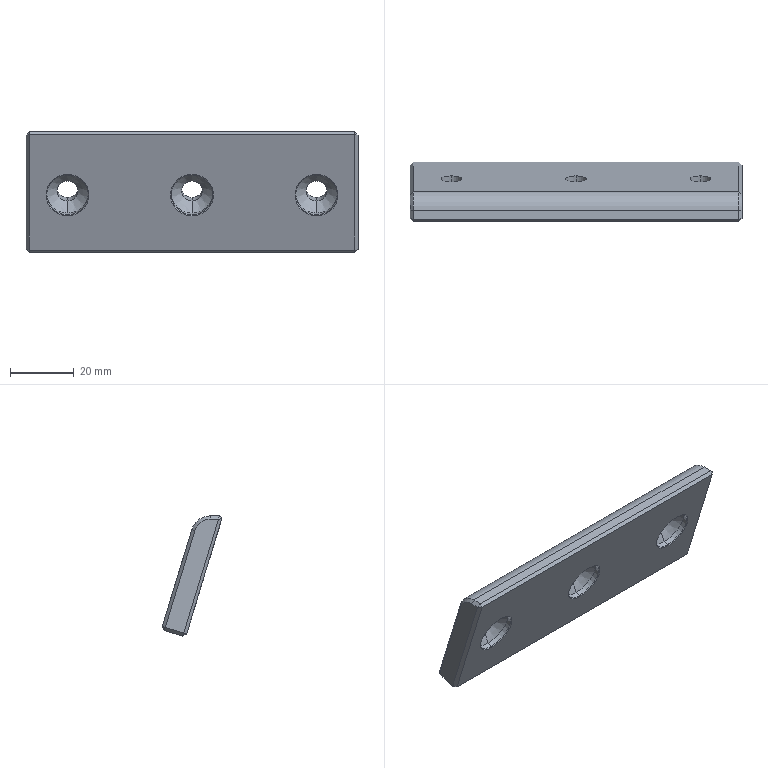Part | Creo | 1 solid | 50 faces | box 104 x 18.672 x 37.672 mm | volume 29709 mm3 | plane 23 | cone 14 | cylinder 13 | commonest cylinder face diameters 6.6 x6 13 x6 12 x1
STEP:
#1=CARTESIAN_POINT('',(0.,0.,0.));
#2=DIRECTION('',(0.,0.,1.));
#3=DIRECTION('',(1.,0.,0.));
#4=AXIS2_PLACEMENT_3D('',#1,#2,#3);
#5=CARTESIAN_POINT('',(38.95,191.692,35.934));
#6=VERTEX_POINT('',#5);
#7=CARTESIAN_POINT('',(38.95,193.621,29.622));
#8=VERTEX_POINT('',#7);
#9=CARTESIAN_POINT('',(38.95,192.656,32.778));
#10=DIRECTION('',(0.,-0.9563,-0.2924));
#11=DIRECTION('',(0.,-0.2924,0.9563));
#12=AXIS2_PLACEMENT_3D('',#9,#10,#11);
#13=CIRCLE('',#12,3.3);
#14=EDGE_CURVE('',#6,#8,#13,.T.);
#15=ORIENTED_EDGE('',*,*,#14,.T.);
#16=CARTESIAN_POINT('',(38.95,190.083,28.54));
#17=VERTEX_POINT('',#16);
#18=CARTESIAN_POINT('',(38.95,190.083,28.54));
#19=DIRECTION('',(0.,0.9563,0.2924));
#20=VECTOR('',#19,3.7);
#21=LINE('',#18,#20);
#22=EDGE_CURVE('',#17,#8,#21,.T.);
#23=ORIENTED_EDGE('',*,*,#22,.F.);
#24=CARTESIAN_POINT('',(38.95,188.153,34.852));
#25=VERTEX_POINT('',#24);
#26=CARTESIAN_POINT('',(38.95,189.118,31.696));
#27=DIRECTION('',(0.,0.9563,0.2924));
#28=DIRECTION('',(0.,0.2924,-0.9563));
#29=AXIS2_PLACEMENT_3D('',#26,#27,#28);
#30=CIRCLE('',#29,3.3);
#31=EDGE_CURVE('',#17,#25,#30,.T.);
#32=ORIENTED_EDGE('',*,*,#31,.T.);
#33=CARTESIAN_POINT('',(38.95,188.153,34.852));
#34=DIRECTION('',(0.,0.9563,0.2924));
#35=VECTOR('',#34,3.7);
#36=LINE('',#33,#35);
#37=EDGE_CURVE('',#25,#6,#36,.T.);
#38=ORIENTED_EDGE('',*,*,#37,.T.);
#39=EDGE_LOOP('',(#15,#23,#32,#38));
#40=FACE_OUTER_BOUND('',#39,.F.);
#41=CARTESIAN_POINT('',(38.95,232.821,45.057));
#42=DIRECTION('',(0.,0.9563,0.2924));
#43=DIRECTION('',(0.,0.2924,-0.9563));
#44=AXIS2_PLACEMENT_3D('',#41,#42,#43);
#45=CYLINDRICAL_SURFACE('',#44,3.3);
#46=ADVANCED_FACE('',(#40),#45,.F.);
#47=CARTESIAN_POINT('',(50.95,188.618,45.987));
#48=VERTEX_POINT('',#47);
#49=CARTESIAN_POINT('',(-51.05,188.618,45.987));
#50=VERTEX_POINT('',#49);
#51=CARTESIAN_POINT('',(50.95,188.618,45.987));
#52=DIRECTION('',(-1.,0.,0.));
#53=VECTOR('',#52,102.);
#54=LINE('',#51,#53);
#55=EDGE_CURVE('',#48,#50,#54,.T.);
#56=ORIENTED_EDGE('',*,*,#55,.T.);
#57=CARTESIAN_POINT('',(-51.05,197.919,15.564));
#58=VERTEX_POINT('',#57);
#59=CARTESIAN_POINT('',(-51.05,197.919,15.564));
#60=DIRECTION('',(0.,-0.2924,0.9563));
#61=VECTOR('',#60,31.813);
#62=LINE('',#59,#61);
#63=EDGE_CURVE('',#58,#50,#62,.T.);
#64=ORIENTED_EDGE('',*,*,#63,.F.);
#65=CARTESIAN_POINT('',(50.95,197.919,15.564));
#66=VERTEX_POINT('',#65);
#67=CARTESIAN_POINT('',(50.95,197.919,15.564));
#68=DIRECTION('',(-1.,0.,0.));
#69=VECTOR('',#68,102.);
#70=LINE('',#67,#69);
#71=EDGE_CURVE('',#66,#58,#70,.T.);
#72=ORIENTED_EDGE('',*,*,#71,.F.);
#73=CARTESIAN_POINT('',(50.95,188.618,45.987));
#74=DIRECTION('',(0.,0.2924,-0.9563));
#75=VECTOR('',#74,31.813);
#76=LINE('',#73,#75);
#77=EDGE_CURVE('',#48,#66,#76,.T.);
#78=ORIENTED_EDGE('',*,*,#77,.F.);
#79=EDGE_LOOP('',(#56,#64,#72,#78));
#80=FACE_OUTER_BOUND('',#79,.F.);
#81=CARTESIAN_POINT('',(-0.05,191.692,35.934));
#82=VERTEX_POINT('',#81);
#83=CARTESIAN_POINT('',(-0.05,193.621,29.622));
#84=VERTEX_POINT('',#83);
#85=CARTESIAN_POINT('',(-0.05,192.656,32.778));
#86=DIRECTION('',(0.,-0.9563,-0.2924));
#87=DIRECTION('',(0.,-0.2924,0.9563));
#88=AXIS2_PLACEMENT_3D('',#85,#86,#87);
#89=CIRCLE('',#88,3.3);
#90=EDGE_CURVE('',#82,#84,#89,.T.);
#91=ORIENTED_EDGE('',*,*,#90,.F.);
#92=CARTESIAN_POINT('',(-0.05,192.656,32.778));
#93=DIRECTION('',(0.,-0.9563,-0.2924));
#94=DIRECTION('',(0.,0.2924,-0.9563));
#95=AXIS2_PLACEMENT_3D('',#92,#93,#94);
#96=CIRCLE('',#95,3.3);
#97=EDGE_CURVE('',#84,#82,#96,.T.);
#98=ORIENTED_EDGE('',*,*,#97,.F.);
#99=EDGE_LOOP('',(#91,#98));
#100=FACE_BOUND('',#99,.F.);
#101=CARTESIAN_POINT('',(-39.05,191.692,35.934));
#102=VERTEX_POINT('',#101);
#103=CARTESIAN_POINT('',(-39.05,193.621,29.622));
#104=VERTEX_POINT('',#103);
#105=CARTESIAN_POINT('',(-39.05,192.656,32.778));
#106=DIRECTION('',(0.,-0.9563,-0.2924));
#107=DIRECTION('',(0.,-0.2924,0.9563));
#108=AXIS2_PLACEMENT_3D('',#105,#106,#107);
#109=CIRCLE('',#108,3.3);
#110=EDGE_CURVE('',#102,#104,#109,.T.);
#111=ORIENTED_EDGE('',*,*,#110,.F.);
#112=CARTESIAN_POINT('',(-39.05,192.656,32.778));
#113=DIRECTION('',(0.,-0.9563,-0.2924));
#114=DIRECTION('',(0.,0.2924,-0.9563));
#115=AXIS2_PLACEMENT_3D('',#112,#113,#114);
#116=CIRCLE('',#115,3.3);
#117=EDGE_CURVE('',#104,#102,#116,.T.);
#118=ORIENTED_EDGE('',*,*,#117,.F.);
#119=EDGE_LOOP('',(#111,#118));
#120=FACE_BOUND('',#119,.F.);
#121=ORIENTED_EDGE('',*,*,#14,.F.);
#122=CARTESIAN_POINT('',(38.95,192.656,32.778));
#123=DIRECTION('',(0.,-0.9563,-0.2924));
#124=DIRECTION('',(0.,0.2924,-0.9563));
#125=AXIS2_PLACEMENT_3D('',#122,#123,#124);
#126=CIRCLE('',#125,3.3);
#127=EDGE_CURVE('',#8,#6,#126,.T.);
#128=ORIENTED_EDGE('',*,*,#127,.F.);
#129=EDGE_LOOP('',(#121,#128));
#130=FACE_BOUND('',#129,.F.);
#131=CARTESIAN_POINT('',(-56.05,205.65,-9.724));
#132=DIRECTION('',(0.,-0.9563,-0.2924));
#133=DIRECTION('',(0.,-0.2924,0.9563));
#134=AXIS2_PLACEMENT_3D('',#131,#132,#133);
#135=PLANE('',#134);
#136=ADVANCED_FACE('',(#80,#100,#120,#130),#135,.F.);
#137=ORIENTED_EDGE('',*,*,#127,.T.);
#138=ORIENTED_EDGE('',*,*,#37,.F.);
#139=CARTESIAN_POINT('',(38.95,189.118,31.696));
#140=DIRECTION('',(0.,0.9563,0.2924));
#141=DIRECTION('',(0.,-0.2924,0.9563));
#142=AXIS2_PLACEMENT_3D('',#139,#140,#141);
#143=CIRCLE('',#142,3.3);
#144=EDGE_CURVE('',#25,#17,#143,.T.);
#145=ORIENTED_EDGE('',*,*,#144,.T.);
#146=ORIENTED_EDGE('',*,*,#22,.T.);
#147=EDGE_LOOP('',(#137,#138,#145,#146));
#148=FACE_OUTER_BOUND('',#147,.F.);
#149=CARTESIAN_POINT('',(38.95,232.821,45.057));
#150=DIRECTION('',(0.,0.9563,0.2924));
#151=DIRECTION('',(0.,0.2924,-0.9563));
#152=AXIS2_PLACEMENT_3D('',#149,#150,#151);
#153=CYLINDRICAL_SURFACE('',#152,3.3);
#154=ADVANCED_FACE('',(#148),#153,.F.);
#155=CARTESIAN_POINT('',(38.95,188.57,24.732));
#156=VERTEX_POINT('',#155);
#157=CARTESIAN_POINT('',(38.95,184.77,37.164));
#158=VERTEX_POINT('',#157);
#159=CARTESIAN_POINT('',(38.95,186.67,30.948));
#160=DIRECTION('',(0.,-0.9563,-0.2924));
#161=DIRECTION('',(0.,0.2924,-0.9563));
#162=AXIS2_PLACEMENT_3D('',#159,#160,#161);
#163=CIRCLE('',#162,6.5);
#164=EDGE_CURVE('',#156,#158,#163,.T.);
#165=ORIENTED_EDGE('',*,*,#164,.F.);
#166=CARTESIAN_POINT('',(38.95,190.083,28.54));
#167=DIRECTION('',(0.,-0.3691,-0.9294));
#168=VECTOR('',#167,4.098);
#169=LINE('',#166,#168);
#170=EDGE_CURVE('',#17,#156,#169,.T.);
#171=ORIENTED_EDGE('',*,*,#170,.F.);
#172=ORIENTED_EDGE('',*,*,#144,.F.);
#173=CARTESIAN_POINT('',(38.95,188.153,34.852));
#174=DIRECTION('',(0.,-0.8257,0.5641));
#175=VECTOR('',#174,4.098);
#176=LINE('',#173,#175);
#177=EDGE_CURVE('',#25,#158,#176,.T.);
#178=ORIENTED_EDGE('',*,*,#177,.T.);
#179=EDGE_LOOP('',(#165,#171,#172,#178));
#180=FACE_OUTER_BOUND('',#179,.F.);
#181=CARTESIAN_POINT('',(38.95,187.894,31.322));
#182=DIRECTION('',(0.,-0.9563,-0.2924));
#183=DIRECTION('',(0.,0.2924,-0.9563));
#184=AXIS2_PLACEMENT_3D('',#181,#182,#183);
#185=CONICAL_SURFACE('',#184,4.9,51.34);
#186=ADVANCED_FACE('',(#180),#185,.F.);
#187=ORIENTED_EDGE('',*,*,#164,.T.);
#188=CARTESIAN_POINT('',(38.95,183.345,36.728));
#189=VERTEX_POINT('',#188);
#190=CARTESIAN_POINT('',(38.95,184.77,37.164));
#191=DIRECTION('',(0.,-0.9563,-0.2924));
#192=VECTOR('',#191,1.49);
#193=LINE('',#190,#192);
#194=EDGE_CURVE('',#158,#189,#193,.T.);
#195=ORIENTED_EDGE('',*,*,#194,.T.);
#196=CARTESIAN_POINT('',(38.95,187.145,24.296));
#197=VERTEX_POINT('',#196);
#198=CARTESIAN_POINT('',(38.95,185.245,30.512));
#199=DIRECTION('',(0.,0.9563,0.2924));
#200=DIRECTION('',(0.,-0.2924,0.9563));
#201=AXIS2_PLACEMENT_3D('',#198,#199,#200);
#202=CIRCLE('',#201,6.5);
#203=EDGE_CURVE('',#189,#197,#202,.T.);
#204=ORIENTED_EDGE('',*,*,#203,.T.);
#205=CARTESIAN_POINT('',(38.95,188.57,24.732));
#206=DIRECTION('',(0.,-0.9563,-0.2924));
#207=VECTOR('',#206,1.49);
#208=LINE('',#205,#207);
#209=EDGE_CURVE('',#156,#197,#208,.T.);
#210=ORIENTED_EDGE('',*,*,#209,.F.);
#211=EDGE_LOOP('',(#187,#195,#204,#210));
#212=FACE_OUTER_BOUND('',#211,.F.);
#213=CARTESIAN_POINT('',(38.95,185.006,30.439));
#214=DIRECTION('',(0.,-0.9563,-0.2924));
#215=DIRECTION('',(0.,0.2924,-0.9563));
#216=AXIS2_PLACEMENT_3D('',#213,#214,#215);
#217=CYLINDRICAL_SURFACE('',#216,6.5);
#218=ADVANCED_FACE('',(#212),#217,.F.);
#219=CARTESIAN_POINT('',(38.95,186.67,30.948));
#220=DIRECTION('',(0.,-0.9563,-0.2924));
#221=DIRECTION('',(0.,-0.2924,0.9563));
#222=AXIS2_PLACEMENT_3D('',#219,#220,#221);
#223=CIRCLE('',#222,6.5);
#224=EDGE_CURVE('',#158,#156,#223,.T.);
#225=ORIENTED_EDGE('',*,*,#224,.T.);
#226=ORIENTED_EDGE('',*,*,#209,.T.);
#227=CARTESIAN_POINT('',(38.95,185.245,30.512));
#228=DIRECTION('',(0.,0.9563,0.2924));
#229=DIRECTION('',(0.,0.2924,-0.9563));
#230=AXIS2_PLACEMENT_3D('',#227,#228,#229);
#231=CIRCLE('',#230,6.5);
#232=EDGE_CURVE('',#197,#189,#231,.T.);
#233=ORIENTED_EDGE('',*,*,#232,.T.);
#234=ORIENTED_EDGE('',*,*,#194,.F.);
#235=EDGE_LOOP('',(#225,#226,#233,#234));
#236=FACE_OUTER_BOUND('',#235,.F.);
#237=CARTESIAN_POINT('',(38.95,185.006,30.439));
#238=DIRECTION('',(0.,-0.9563,-0.2924));
#239=DIRECTION('',(0.,0.2924,-0.9563));
#240=AXIS2_PLACEMENT_3D('',#237,#238,#239);
#241=CYLINDRICAL_SURFACE('',#240,6.5);
#242=ADVANCED_FACE('',(#236),#241,.F.);
#243=ORIENTED_EDGE('',*,*,#224,.F.);
#244=ORIENTED_EDGE('',*,*,#177,.F.);
#245=ORIENTED_EDGE('',*,*,#31,.F.);
#246=ORIENTED_EDGE('',*,*,#170,.T.);
#247=EDGE_LOOP('',(#243,#244,#245,#246));
#248=FACE_OUTER_BOUND('',#247,.F.);
#249=CARTESIAN_POINT('',(38.95,187.894,31.322));
#250=DIRECTION('',(0.,-0.9563,-0.2924));
#251=DIRECTION('',(0.,0.2924,-0.9563));
#252=AXIS2_PLACEMENT_3D('',#249,#250,#251);
#253=CONICAL_SURFACE('',#252,4.9,51.34);
#254=ADVANCED_FACE('',(#248),#253,.F.);
#255=CARTESIAN_POINT('',(38.95,186.979,23.984));
#256=VERTEX_POINT('',#255);
#257=CARTESIAN_POINT('',(38.95,183.032,36.894));
#258=VERTEX_POINT('',#257);
#259=CARTESIAN_POINT('',(38.95,185.006,30.439));
#260=DIRECTION('',(0.,0.9563,0.2924));
#261=DIRECTION('',(0.,0.2924,-0.9563));
#262=AXIS2_PLACEMENT_3D('',#259,#260,#261);
#263=CIRCLE('',#262,6.75);
#264=EDGE_CURVE('',#256,#258,#263,.T.);
#265=ORIENTED_EDGE('',*,*,#264,.T.);
#266=CARTESIAN_POINT('',(38.95,183.345,36.728));
#267=DIRECTION('',(0.,-0.8829,0.4695));
#268=VECTOR('',#267,0.3536);
#269=LINE('',#266,#268);
#270=EDGE_CURVE('',#189,#258,#269,.T.);
#271=ORIENTED_EDGE('',*,*,#270,.F.);
#272=ORIENTED_EDGE('',*,*,#232,.F.);
#273=CARTESIAN_POINT('',(38.95,187.145,24.296));
#274=DIRECTION('',(0.,-0.4695,-0.8829));
#275=VECTOR('',#274,0.3536);
#276=LINE('',#273,#275);
#277=EDGE_CURVE('',#197,#256,#276,.T.);
#278=ORIENTED_EDGE('',*,*,#277,.T.);
#279=EDGE_LOOP('',(#265,#271,#272,#278));
#280=FACE_OUTER_BOUND('',#279,.F.);
#281=CARTESIAN_POINT('',(38.95,185.126,30.475));
#282=DIRECTION('',(0.,-0.9563,-0.2924));
#283=DIRECTION('',(0.,-0.2924,0.9563));
#284=AXIS2_PLACEMENT_3D('',#281,#282,#283);
#285=CONICAL_SURFACE('',#284,6.625,45.);
#286=ADVANCED_FACE('',(#280),#285,.F.);
#287=CARTESIAN_POINT('',(50.95,190.269,13.225));
#288=VERTEX_POINT('',#287);
#289=CARTESIAN_POINT('',(50.95,179.247,49.277));
#290=VERTEX_POINT('',#289);
#291=CARTESIAN_POINT('',(50.95,190.269,13.225));
#292=DIRECTION('',(0.,-0.2924,0.9563));
#293=VECTOR('',#292,37.699);
#294=LINE('',#291,#293);
#295=EDGE_CURVE('',#288,#290,#294,.T.);
#296=ORIENTED_EDGE('',*,*,#295,.F.);
#297=CARTESIAN_POINT('',(-51.05,190.269,13.225));
#298=VERTEX_POINT('',#297);
#299=CARTESIAN_POINT('',(-51.05,190.269,13.225));
#300=DIRECTION('',(1.,0.,0.));
#301=VECTOR('',#300,102.);
#302=LINE('',#299,#301);
#303=EDGE_CURVE('',#298,#288,#302,.T.);
#304=ORIENTED_EDGE('',*,*,#303,.F.);
#305=CARTESIAN_POINT('',(-51.05,179.247,49.277));
#306=VERTEX_POINT('',#305);
#307=CARTESIAN_POINT('',(-51.05,179.247,49.277));
#308=DIRECTION('',(0.,0.2924,-0.9563));
#309=VECTOR('',#308,37.699);
#310=LINE('',#307,#309);
#311=EDGE_CURVE('',#306,#298,#310,.T.);
#312=ORIENTED_EDGE('',*,*,#311,.F.);
#313=CARTESIAN_POINT('',(50.95,179.247,49.277));
#314=DIRECTION('',(-1.,0.,0.));
#315=VECTOR('',#314,102.);
#316=LINE('',#313,#315);
#317=EDGE_CURVE('',#290,#306,#316,.T.);
#318=ORIENTED_EDGE('',*,*,#317,.F.);
#319=EDGE_LOOP('',(#296,#304,#312,#318));
#320=FACE_OUTER_BOUND('',#319,.F.);
#321=ORIENTED_EDGE('',*,*,#264,.F.);
#322=CARTESIAN_POINT('',(38.95,185.006,30.439));
#323=DIRECTION('',(0.,0.9563,0.2924));
#324=DIRECTION('',(0.,-0.2924,0.9563));
#325=AXIS2_PLACEMENT_3D('',#322,#323,#324);
#326=CIRCLE('',#325,6.75);
#327=EDGE_CURVE('',#258,#256,#326,.T.);
#328=ORIENTED_EDGE('',*,*,#327,.F.);
#329=EDGE_LOOP('',(#321,#328));
#330=FACE_BOUND('',#329,.F.);
#331=CARTESIAN_POINT('',(-0.05,186.979,23.984));
#332=VERTEX_POINT('',#331);
#333=CARTESIAN_POINT('',(-0.05,183.032,36.894));
#334=VERTEX_POINT('',#333);
#335=CARTESIAN_POINT('',(-0.05,185.006,30.439));
#336=DIRECTION('',(0.,0.9563,0.2924));
#337=DIRECTION('',(0.,0.2924,-0.9563));
#338=AXIS2_PLACEMENT_3D('',#335,#336,#337);
#339=CIRCLE('',#338,6.75);
#340=EDGE_CURVE('',#332,#334,#339,.T.);
#341=ORIENTED_EDGE('',*,*,#340,.F.);
#342=CARTESIAN_POINT('',(-0.05,185.006,30.439));
#343=DIRECTION('',(0.,0.9563,0.2924));
#344=DIRECTION('',(0.,-0.2924,0.9563));
#345=AXIS2_PLACEMENT_3D('',#342,#343,#344);
#346=CIRCLE('',#345,6.75);
#347=EDGE_CURVE('',#334,#332,#346,.T.);
#348=ORIENTED_EDGE('',*,*,#347,.F.);
#349=EDGE_LOOP('',(#341,#348));
#350=FACE_BOUND('',#349,.F.);
#351=CARTESIAN_POINT('',(-39.05,186.979,23.984));
#352=VERTEX_POINT('',#351);
#353=CARTESIAN_POINT('',(-39.05,183.032,36.894));
#354=VERTEX_POINT('',#353);
#355=CARTESIAN_POINT('',(-39.05,185.006,30.439));
#356=DIRECTION('',(0.,0.9563,0.2924));
#357=DIRECTION('',(0.,0.2924,-0.9563));
#358=AXIS2_PLACEMENT_3D('',#355,#356,#357);
#359=CIRCLE('',#358,6.75);
#360=EDGE_CURVE('',#352,#354,#359,.T.);
#361=ORIENTED_EDGE('',*,*,#360,.F.);
#362=CARTESIAN_POINT('',(-39.05,185.006,30.439));
#363=DIRECTION('',(0.,0.9563,0.2924));
#364=DIRECTION('',(0.,-0.2924,0.9563));
#365=AXIS2_PLACEMENT_3D('',#362,#363,#364);
#366=CIRCLE('',#365,6.75);
#367=EDGE_CURVE('',#354,#352,#366,.T.);
#368=ORIENTED_EDGE('',*,*,#367,.F.);
#369=EDGE_LOOP('',(#361,#368));
#370=FACE_BOUND('',#369,.F.);
#371=CARTESIAN_POINT('',(-56.05,198.,-12.063));
#372=DIRECTION('',(0.,-0.9563,-0.2924));
#373=DIRECTION('',(0.,-0.2924,0.9563));
#374=AXIS2_PLACEMENT_3D('',#371,#372,#373);
#375=PLANE('',#374);
#376=ADVANCED_FACE('',(#320,#330,#350,#370),#375,.T.);
#377=CARTESIAN_POINT('',(51.95,180.306,49.233));
#378=VERTEX_POINT('',#377);
#379=CARTESIAN_POINT('',(51.95,180.306,49.233));
#380=DIRECTION('',(-0.6862,-0.7268,0.02999));
#381=VECTOR('',#380,1.457);
#382=LINE('',#379,#381);
#383=EDGE_CURVE('',#378,#290,#382,.T.);
#384=ORIENTED_EDGE('',*,*,#383,.F.);
#385=CARTESIAN_POINT('',(51.95,191.225,13.518));
#386=VERTEX_POINT('',#385);
#387=CARTESIAN_POINT('',(51.95,180.306,49.233));
#388=DIRECTION('',(0.,0.2924,-0.9563));
#389=VECTOR('',#388,37.347);
#390=LINE('',#387,#389);
#391=EDGE_CURVE('',#378,#386,#390,.T.);
#392=ORIENTED_EDGE('',*,*,#391,.T.);
#393=CARTESIAN_POINT('',(51.95,191.225,13.518));
#394=DIRECTION('',(-0.7071,-0.6762,-0.2067));
#395=VECTOR('',#394,1.414);
#396=LINE('',#393,#395);
#397=EDGE_CURVE('',#386,#288,#396,.T.);
#398=ORIENTED_EDGE('',*,*,#397,.T.);
#399=ORIENTED_EDGE('',*,*,#295,.T.);
#400=EDGE_LOOP('',(#384,#392,#398,#399));
#401=FACE_OUTER_BOUND('',#400,.F.);
#402=CARTESIAN_POINT('',(50.95,198.,-12.063));
#403=DIRECTION('',(0.7071,-0.6762,-0.2067));
#404=DIRECTION('',(0.,-0.2924,0.9563));
#405=AXIS2_PLACEMENT_3D('',#402,#403,#404);
#406=PLANE('',#405);
#407=ADVANCED_FACE('',(#401),#406,.T.);
#408=CARTESIAN_POINT('',(50.95,179.954,50.233));
#409=VERTEX_POINT('',#408);
#410=CARTESIAN_POINT('',(50.95,179.954,50.233));
#411=DIRECTION('',(0.,-0.5948,-0.8039));
#412=VECTOR('',#411,1.19);
#413=LINE('',#410,#412);
#414=EDGE_CURVE('',#409,#290,#413,.T.);
#415=ORIENTED_EDGE('',*,*,#414,.F.);
#416=CARTESIAN_POINT('',(51.95,180.306,49.233));
#417=DIRECTION('',(-0.6862,-0.2412,0.6862));
#418=VECTOR('',#417,1.457);
#419=LINE('',#416,#418);
#420=EDGE_CURVE('',#378,#409,#419,.T.);
#421=ORIENTED_EDGE('',*,*,#420,.F.);
#422=ORIENTED_EDGE('',*,*,#383,.T.);
#423=EDGE_LOOP('',(#415,#421,#422));
#424=FACE_OUTER_BOUND('',#423,.F.);
#425=CARTESIAN_POINT('',(50.95,179.954,50.233));
#426=DIRECTION('',(0.6595,-0.6043,0.4471));
#427=DIRECTION('',(-0.6756,-0.7373,0.));
#428=AXIS2_PLACEMENT_3D('',#425,#426,#427);
#429=PLANE('',#428);
#430=ADVANCED_FACE('',(#424),#429,.T.);
#431=CARTESIAN_POINT('',(-51.05,179.954,50.233));
#432=VERTEX_POINT('',#431);
#433=CARTESIAN_POINT('',(-51.05,179.247,49.277));
#434=DIRECTION('',(0.,0.5948,0.8039));
#435=VECTOR('',#434,1.19);
#436=LINE('',#433,#435);
#437=EDGE_CURVE('',#306,#432,#436,.T.);
#438=ORIENTED_EDGE('',*,*,#437,.T.);
#439=CARTESIAN_POINT('',(-51.05,179.954,50.233));
#440=DIRECTION('',(1.,0.,0.));
#441=VECTOR('',#440,102.);
#442=LINE('',#439,#441);
#443=EDGE_CURVE('',#432,#409,#442,.T.);
#444=ORIENTED_EDGE('',*,*,#443,.T.);
#445=ORIENTED_EDGE('',*,*,#414,.T.);
#446=ORIENTED_EDGE('',*,*,#317,.T.);
#447=EDGE_LOOP('',(#438,#444,#445,#446));
#448=FACE_OUTER_BOUND('',#447,.F.);
#449=CARTESIAN_POINT('',(-56.05,179.247,49.277));
#450=DIRECTION('',(0.,-0.8039,0.5948));
#451=DIRECTION('',(-1.,0.,0.));
#452=AXIS2_PLACEMENT_3D('',#449,#450,#451);
#453=PLANE('',#452);
#454=ADVANCED_FACE('',(#448),#453,.T.);
#455=CARTESIAN_POINT('',(-52.05,180.306,49.233));
#456=VERTEX_POINT('',#455);
#457=CARTESIAN_POINT('',(-51.05,179.247,49.277));
#458=DIRECTION('',(-0.6862,0.7268,-0.02999));
#459=VECTOR('',#458,1.457);
#460=LINE('',#457,#459);
#461=EDGE_CURVE('',#306,#456,#460,.T.);
#462=ORIENTED_EDGE('',*,*,#461,.T.);
#463=CARTESIAN_POINT('',(-51.05,179.954,50.233));
#464=DIRECTION('',(-0.6862,0.2412,-0.6862));
#465=VECTOR('',#464,1.457);
#466=LINE('',#463,#465);
#467=EDGE_CURVE('',#432,#456,#466,.T.);
#468=ORIENTED_EDGE('',*,*,#467,.F.);
#469=ORIENTED_EDGE('',*,*,#437,.F.);
#470=EDGE_LOOP('',(#462,#468,#469));
#471=FACE_OUTER_BOUND('',#470,.F.);
#472=CARTESIAN_POINT('',(-52.05,180.306,49.233));
#473=DIRECTION('',(-0.6595,-0.6043,0.4471));
#474=DIRECTION('',(-0.6756,0.7373,0.));
#475=AXIS2_PLACEMENT_3D('',#472,#473,#474);
#476=PLANE('',#475);
#477=ADVANCED_FACE('',(#471),#476,.T.);
#478=ORIENTED_EDGE('',*,*,#461,.F.);
#479=ORIENTED_EDGE('',*,*,#311,.T.);
#480=CARTESIAN_POINT('',(-52.05,191.225,13.518));
#481=VERTEX_POINT('',#480);
#482=CARTESIAN_POINT('',(-51.05,190.269,13.225));
#483=DIRECTION('',(-0.7071,0.6762,0.2067));
#484=VECTOR('',#483,1.414);
#485=LINE('',#482,#484);
#486=EDGE_CURVE('',#298,#481,#485,.T.);
#487=ORIENTED_EDGE('',*,*,#486,.T.);
#488=CARTESIAN_POINT('',(-52.05,191.225,13.518));
#489=DIRECTION('',(0.,-0.2924,0.9563));
#490=VECTOR('',#489,37.347);
#491=LINE('',#488,#490);
#492=EDGE_CURVE('',#481,#456,#491,.T.);
#493=ORIENTED_EDGE('',*,*,#492,.T.);
#494=EDGE_LOOP('',(#478,#479,#487,#493));
#495=FACE_OUTER_BOUND('',#494,.F.);
#496=CARTESIAN_POINT('',(-51.05,198.,-12.063));
#497=DIRECTION('',(0.7071,0.6762,0.2067));
#498=DIRECTION('',(0.,-0.2924,0.9563));
#499=AXIS2_PLACEMENT_3D('',#496,#497,#498);
#500=PLANE('',#499);
#501=ADVANCED_FACE('',(#495),#500,.F.);
#502=CARTESIAN_POINT('',(-51.05,191.517,12.561));
#503=VERTEX_POINT('',#502);
#504=CARTESIAN_POINT('',(-52.05,191.225,13.518));
#505=DIRECTION('',(0.7071,0.2067,-0.6762));
#506=VECTOR('',#505,1.414);
#507=LINE('',#504,#506);
#508=EDGE_CURVE('',#481,#503,#507,.T.);
#509=ORIENTED_EDGE('',*,*,#508,.F.);
#510=ORIENTED_EDGE('',*,*,#486,.F.);
#511=CARTESIAN_POINT('',(-51.05,191.517,12.561));
#512=DIRECTION('',(0.,-0.8829,0.4695));
#513=VECTOR('',#512,1.414);
#514=LINE('',#511,#513);
#515=EDGE_CURVE('',#503,#298,#514,.T.);
#516=ORIENTED_EDGE('',*,*,#515,.F.);
#517=EDGE_LOOP('',(#509,#510,#516));
#518=FACE_OUTER_BOUND('',#517,.F.);
#519=CARTESIAN_POINT('',(-51.05,190.269,13.225));
#520=DIRECTION('',(-0.5774,-0.3833,-0.7209));
#521=DIRECTION('',(-0.7805,0.,0.6251));
#522=AXIS2_PLACEMENT_3D('',#519,#520,#521);
#523=PLANE('',#522);
#524=ADVANCED_FACE('',(#518),#523,.T.);
#525=CARTESIAN_POINT('',(-51.05,197.255,14.316));
#526=VERTEX_POINT('',#525);
#527=CARTESIAN_POINT('',(-52.05,196.963,15.272));
#528=VERTEX_POINT('',#527);
#529=CARTESIAN_POINT('',(-51.05,197.255,14.316));
#530=DIRECTION('',(-0.7071,-0.2067,0.6762));
#531=VECTOR('',#530,1.414);
#532=LINE('',#529,#531);
#533=EDGE_CURVE('',#526,#528,#532,.T.);
#534=ORIENTED_EDGE('',*,*,#533,.T.);
#535=CARTESIAN_POINT('',(-52.05,196.963,15.272));
#536=DIRECTION('',(0.,-0.9563,-0.2924));
#537=VECTOR('',#536,6.);
#538=LINE('',#535,#537);
#539=EDGE_CURVE('',#528,#481,#538,.T.);
#540=ORIENTED_EDGE('',*,*,#539,.T.);
#541=ORIENTED_EDGE('',*,*,#508,.T.);
#542=CARTESIAN_POINT('',(-51.05,191.517,12.561));
#543=DIRECTION('',(0.,0.9563,0.2924));
#544=VECTOR('',#543,6.);
#545=LINE('',#542,#544);
#546=EDGE_CURVE('',#503,#526,#545,.T.);
#547=ORIENTED_EDGE('',*,*,#546,.T.);
#548=EDGE_LOOP('',(#534,#540,#541,#547));
#549=FACE_OUTER_BOUND('',#548,.F.);
#550=CARTESIAN_POINT('',(-52.05,190.269,13.225));
#551=DIRECTION('',(0.7071,-0.2067,0.6762));
#552=DIRECTION('',(0.,0.9563,0.2924));
#553=AXIS2_PLACEMENT_3D('',#550,#551,#552);
#554=PLANE('',#553);
#555=ADVANCED_FACE('',(#549),#554,.F.);
#556=CARTESIAN_POINT('',(-52.05,196.963,15.272));
#557=DIRECTION('',(0.7071,0.6762,0.2067));
#558=VECTOR('',#557,1.414);
#559=LINE('',#556,#558);
#560=EDGE_CURVE('',#528,#58,#559,.T.);
#561=ORIENTED_EDGE('',*,*,#560,.F.);
#562=ORIENTED_EDGE('',*,*,#533,.F.);
#563=CARTESIAN_POINT('',(-51.05,197.919,15.564));
#564=DIRECTION('',(0.,-0.4695,-0.8829));
#565=VECTOR('',#564,1.414);
#566=LINE('',#563,#565);
#567=EDGE_CURVE('',#58,#526,#566,.T.);
#568=ORIENTED_EDGE('',*,*,#567,.F.);
#569=EDGE_LOOP('',(#561,#562,#568));
#570=FACE_OUTER_BOUND('',#569,.F.);
#571=CARTESIAN_POINT('',(-51.05,197.919,15.564));
#572=DIRECTION('',(-0.5774,0.7209,-0.3833));
#573=DIRECTION('',(0.7805,0.6251,0.));
#574=AXIS2_PLACEMENT_3D('',#571,#572,#573);
#575=PLANE('',#574);
#576=ADVANCED_FACE('',(#570),#575,.T.);
#577=CARTESIAN_POINT('',(-52.05,187.662,45.695));
#578=VERTEX_POINT('',#577);
#579=CARTESIAN_POINT('',(-51.05,188.618,45.987));
#580=DIRECTION('',(-0.7071,-0.6762,-0.2067));
#581=VECTOR('',#580,1.414);
#582=LINE('',#579,#581);
#583=EDGE_CURVE('',#50,#578,#582,.T.);
#584=ORIENTED_EDGE('',*,*,#583,.T.);
#585=CARTESIAN_POINT('',(-52.05,187.662,45.695));
#586=DIRECTION('',(0.,0.2924,-0.9563));
#587=VECTOR('',#586,31.813);
#588=LINE('',#585,#587);
#589=EDGE_CURVE('',#578,#528,#588,.T.);
#590=ORIENTED_EDGE('',*,*,#589,.T.);
#591=ORIENTED_EDGE('',*,*,#560,.T.);
#592=ORIENTED_EDGE('',*,*,#63,.T.);
#593=EDGE_LOOP('',(#584,#590,#591,#592));
#594=FACE_OUTER_BOUND('',#593,.F.);
#595=CARTESIAN_POINT('',(-52.05,187.379,46.619));
#596=DIRECTION('',(-0.7071,0.6762,0.2067));
#597=DIRECTION('',(0.,0.2924,-0.9563));
#598=AXIS2_PLACEMENT_3D('',#595,#596,#597);
#599=PLANE('',#598);
#600=ADVANCED_FACE('',(#594),#599,.T.);
#601=CARTESIAN_POINT('',(-52.05,182.88,49.233));
#602=VERTEX_POINT('',#601);
#603=CARTESIAN_POINT('',(-51.05,182.88,50.233));
#604=VERTEX_POINT('',#603);
#605=CARTESIAN_POINT('',(-52.05,182.88,49.233));
#606=DIRECTION('',(0.7071,0.,0.7071));
#607=VECTOR('',#606,1.414);
#608=LINE('',#605,#607);
#609=EDGE_CURVE('',#602,#604,#608,.T.);
#610=ORIENTED_EDGE('',*,*,#609,.F.);
#611=CARTESIAN_POINT('',(-52.05,182.88,44.233));
#612=DIRECTION('',(-1.,0.,0.));
#613=DIRECTION('',(0.,0.,1.));
#614=AXIS2_PLACEMENT_3D('',#611,#612,#613);
#615=CIRCLE('',#614,5.);
#616=EDGE_CURVE('',#602,#578,#615,.T.);
#617=ORIENTED_EDGE('',*,*,#616,.T.);
#618=ORIENTED_EDGE('',*,*,#583,.F.);
#619=CARTESIAN_POINT('',(-51.05,182.88,44.233));
#620=DIRECTION('',(-1.,0.,0.));
#621=DIRECTION('',(0.,0.,1.));
#622=AXIS2_PLACEMENT_3D('',#619,#620,#621);
#623=CIRCLE('',#622,6.);
#624=EDGE_CURVE('',#604,#50,#623,.T.);
#625=ORIENTED_EDGE('',*,*,#624,.F.);
#626=EDGE_LOOP('',(#610,#617,#618,#625));
#627=FACE_OUTER_BOUND('',#626,.F.);
#628=CARTESIAN_POINT('',(-51.55,182.88,44.233));
#629=DIRECTION('',(1.,0.,0.));
#630=DIRECTION('',(0.,0.,-1.));
#631=AXIS2_PLACEMENT_3D('',#628,#629,#630);
#632=CONICAL_SURFACE('',#631,5.5,45.);
#633=ADVANCED_FACE('',(#627),#632,.T.);
#634=ORIENTED_EDGE('',*,*,#467,.T.);
#635=CARTESIAN_POINT('',(-52.05,180.306,49.233));
#636=DIRECTION('',(0.,1.,0.));
#637=VECTOR('',#636,2.574);
#638=LINE('',#635,#637);
#639=EDGE_CURVE('',#456,#602,#638,.T.);
#640=ORIENTED_EDGE('',*,*,#639,.T.);
#641=ORIENTED_EDGE('',*,*,#609,.T.);
#642=CARTESIAN_POINT('',(-51.05,182.88,50.233));
#643=DIRECTION('',(0.,-1.,0.));
#644=VECTOR('',#643,2.926);
#645=LINE('',#642,#644);
#646=EDGE_CURVE('',#604,#432,#645,.T.);
#647=ORIENTED_EDGE('',*,*,#646,.T.);
#648=EDGE_LOOP('',(#634,#640,#641,#647));
#649=FACE_OUTER_BOUND('',#648,.F.);
#650=CARTESIAN_POINT('',(-51.05,168.954,50.233));
#651=DIRECTION('',(-0.7071,0.,0.7071));
#652=DIRECTION('',(0.,-1.,0.));
#653=AXIS2_PLACEMENT_3D('',#650,#651,#652);
#654=PLANE('',#653);
#655=ADVANCED_FACE('',(#649),#654,.T.);
#656=ORIENTED_EDGE('',*,*,#589,.F.);
#657=ORIENTED_EDGE('',*,*,#616,.F.);
#658=ORIENTED_EDGE('',*,*,#639,.F.);
#659=ORIENTED_EDGE('',*,*,#492,.F.);
#660=ORIENTED_EDGE('',*,*,#539,.F.);
#661=EDGE_LOOP('',(#656,#657,#658,#659,#660));
#662=FACE_OUTER_BOUND('',#661,.F.);
#663=CARTESIAN_POINT('',(-52.05,180.685,44.572));
#664=DIRECTION('',(-1.,0.,0.));
#665=DIRECTION('',(0.,-0.2924,0.9563));
#666=AXIS2_PLACEMENT_3D('',#663,#664,#665);
#667=PLANE('',#666);
#668=ADVANCED_FACE('',(#662),#667,.T.);
#669=ORIENTED_EDGE('',*,*,#443,.F.);
#670=ORIENTED_EDGE('',*,*,#646,.F.);
#671=CARTESIAN_POINT('',(50.95,182.88,50.233));
#672=VERTEX_POINT('',#671);
#673=CARTESIAN_POINT('',(-51.05,182.88,50.233));
#674=DIRECTION('',(1.,0.,0.));
#675=VECTOR('',#674,102.);
#676=LINE('',#673,#675);
#677=EDGE_CURVE('',#604,#672,#676,.T.);
#678=ORIENTED_EDGE('',*,*,#677,.T.);
#679=CARTESIAN_POINT('',(50.95,179.954,50.233));
#680=DIRECTION('',(0.,1.,0.));
#681=VECTOR('',#680,2.926);
#682=LINE('',#679,#681);
#683=EDGE_CURVE('',#409,#672,#682,.T.);
#684=ORIENTED_EDGE('',*,*,#683,.F.);
#685=EDGE_LOOP('',(#669,#670,#678,#684));
#686=FACE_OUTER_BOUND('',#685,.F.);
#687=CARTESIAN_POINT('',(-56.05,168.954,50.233));
#688=DIRECTION('',(0.,0.,-1.));
#689=DIRECTION('',(0.,-1.,0.));
#690=AXIS2_PLACEMENT_3D('',#687,#688,#689);
#691=PLANE('',#690);
#692=ADVANCED_FACE('',(#686),#691,.F.);
#693=ORIENTED_EDGE('',*,*,#677,.F.);
#694=ORIENTED_EDGE('',*,*,#624,.T.);
#695=ORIENTED_EDGE('',*,*,#55,.F.);
#696=CARTESIAN_POINT('',(50.95,182.88,44.233));
#697=DIRECTION('',(1.,0.,0.));
#698=DIRECTION('',(0.,0.9563,0.2924));
#699=AXIS2_PLACEMENT_3D('',#696,#697,#698);
#700=CIRCLE('',#699,6.);
#701=EDGE_CURVE('',#48,#672,#700,.T.);
#702=ORIENTED_EDGE('',*,*,#701,.T.);
#703=EDGE_LOOP('',(#693,#694,#695,#702));
#704=FACE_OUTER_BOUND('',#703,.F.);
#705=CARTESIAN_POINT('',(-56.05,182.88,44.233));
#706=DIRECTION('',(1.,0.,0.));
#707=DIRECTION('',(0.,0.,-1.));
#708=AXIS2_PLACEMENT_3D('',#705,#706,#707);
#709=CYLINDRICAL_SURFACE('',#708,6.);
#710=ADVANCED_FACE('',(#704),#709,.T.);
#711=CARTESIAN_POINT('',(51.95,182.88,49.233));
#712=VERTEX_POINT('',#711);
#713=CARTESIAN_POINT('',(50.95,182.88,50.233));
#714=DIRECTION('',(0.7071,0.,-0.7071));
#715=VECTOR('',#714,1.414);
#716=LINE('',#713,#715);
#717=EDGE_CURVE('',#672,#712,#716,.T.);
#718=ORIENTED_EDGE('',*,*,#717,.F.);
#719=ORIENTED_EDGE('',*,*,#701,.F.);
#720=CARTESIAN_POINT('',(51.95,187.662,45.695));
#721=VERTEX_POINT('',#720);
#722=CARTESIAN_POINT('',(51.95,187.662,45.695));
#723=DIRECTION('',(-0.7071,0.6762,0.2067));
#724=VECTOR('',#723,1.414);
#725=LINE('',#722,#724);
#726=EDGE_CURVE('',#721,#48,#725,.T.);
#727=ORIENTED_EDGE('',*,*,#726,.F.);
#728=CARTESIAN_POINT('',(51.95,182.88,44.233));
#729=DIRECTION('',(1.,0.,0.));
#730=DIRECTION('',(0.,0.9563,0.2924));
#731=AXIS2_PLACEMENT_3D('',#728,#729,#730);
#732=CIRCLE('',#731,5.);
#733=EDGE_CURVE('',#721,#712,#732,.T.);
#734=ORIENTED_EDGE('',*,*,#733,.T.);
#735=EDGE_LOOP('',(#718,#719,#727,#734));
#736=FACE_OUTER_BOUND('',#735,.F.);
#737=CARTESIAN_POINT('',(51.45,182.88,44.233));
#738=DIRECTION('',(-1.,0.,0.));
#739=DIRECTION('',(0.,0.,1.));
#740=AXIS2_PLACEMENT_3D('',#737,#738,#739);
#741=CONICAL_SURFACE('',#740,5.5,45.);
#742=ADVANCED_FACE('',(#736),#741,.T.);
#743=ORIENTED_EDGE('',*,*,#420,.T.);
#744=ORIENTED_EDGE('',*,*,#683,.T.);
#745=ORIENTED_EDGE('',*,*,#717,.T.);
#746=CARTESIAN_POINT('',(51.95,182.88,49.233));
#747=DIRECTION('',(0.,-1.,0.));
#748=VECTOR('',#747,2.574);
#749=LINE('',#746,#748);
#750=EDGE_CURVE('',#712,#378,#749,.T.);
#751=ORIENTED_EDGE('',*,*,#750,.T.);
#752=EDGE_LOOP('',(#743,#744,#745,#751));
#753=FACE_OUTER_BOUND('',#752,.F.);
#754=CARTESIAN_POINT('',(51.95,198.,49.233));
#755=DIRECTION('',(-0.7071,0.,-0.7071));
#756=DIRECTION('',(0.,1.,0.));
#757=AXIS2_PLACEMENT_3D('',#754,#755,#756);
#758=PLANE('',#757);
#759=ADVANCED_FACE('',(#753),#758,.F.);
#760=ORIENTED_EDGE('',*,*,#391,.F.);
#761=ORIENTED_EDGE('',*,*,#750,.F.);
#762=ORIENTED_EDGE('',*,*,#733,.F.);
#763=CARTESIAN_POINT('',(51.95,196.963,15.272));
#764=VERTEX_POINT('',#763);
#765=CARTESIAN_POINT('',(51.95,196.963,15.272));
#766=DIRECTION('',(0.,-0.2924,0.9563));
#767=VECTOR('',#766,31.813);
#768=LINE('',#765,#767);
#769=EDGE_CURVE('',#764,#721,#768,.T.);
#770=ORIENTED_EDGE('',*,*,#769,.F.);
#771=CARTESIAN_POINT('',(51.95,191.225,13.518));
#772=DIRECTION('',(0.,0.9563,0.2924));
#773=VECTOR('',#772,6.);
#774=LINE('',#771,#773);
#775=EDGE_CURVE('',#386,#764,#774,.T.);
#776=ORIENTED_EDGE('',*,*,#775,.F.);
#777=EDGE_LOOP('',(#760,#761,#762,#770,#776));
#778=FACE_OUTER_BOUND('',#777,.F.);
#779=CARTESIAN_POINT('',(51.95,198.,-12.063));
#780=DIRECTION('',(-1.,0.,0.));
#781=DIRECTION('',(0.,-0.2924,0.9563));
#782=AXIS2_PLACEMENT_3D('',#779,#780,#781);
#783=PLANE('',#782);
#784=ADVANCED_FACE('',(#778),#783,.F.);
#785=ORIENTED_EDGE('',*,*,#726,.T.);
#786=ORIENTED_EDGE('',*,*,#77,.T.);
#787=CARTESIAN_POINT('',(50.95,197.919,15.564));
#788=DIRECTION('',(0.7071,-0.6762,-0.2067));
#789=VECTOR('',#788,1.414);
#790=LINE('',#787,#789);
#791=EDGE_CURVE('',#66,#764,#790,.T.);
#792=ORIENTED_EDGE('',*,*,#791,.T.);
#793=ORIENTED_EDGE('',*,*,#769,.T.);
#794=EDGE_LOOP('',(#785,#786,#792,#793));
#795=FACE_OUTER_BOUND('',#794,.F.);
#796=CARTESIAN_POINT('',(51.95,204.694,-10.016));
#797=DIRECTION('',(-0.7071,-0.6762,-0.2067));
#798=DIRECTION('',(0.,0.2924,-0.9563));
#799=AXIS2_PLACEMENT_3D('',#796,#797,#798);
#800=PLANE('',#799);
#801=ADVANCED_FACE('',(#795),#800,.F.);
#802=ORIENTED_EDGE('',*,*,#791,.F.);
#803=CARTESIAN_POINT('',(50.95,197.255,14.316));
#804=VERTEX_POINT('',#803);
#805=CARTESIAN_POINT('',(50.95,197.255,14.316));
#806=DIRECTION('',(0.,0.4695,0.8829));
#807=VECTOR('',#806,1.414);
#808=LINE('',#805,#807);
#809=EDGE_CURVE('',#804,#66,#808,.T.);
#810=ORIENTED_EDGE('',*,*,#809,.F.);
#811=CARTESIAN_POINT('',(51.95,196.963,15.272));
#812=DIRECTION('',(-0.7071,0.2067,-0.6762));
#813=VECTOR('',#812,1.414);
#814=LINE('',#811,#813);
#815=EDGE_CURVE('',#764,#804,#814,.T.);
#816=ORIENTED_EDGE('',*,*,#815,.F.);
#817=EDGE_LOOP('',(#802,#810,#816));
#818=FACE_OUTER_BOUND('',#817,.F.);
#819=CARTESIAN_POINT('',(50.95,197.255,14.316));
#820=DIRECTION('',(0.5774,0.7209,-0.3833));
#821=DIRECTION('',(0.7805,-0.6251,0.));
#822=AXIS2_PLACEMENT_3D('',#819,#820,#821);
#823=PLANE('',#822);
#824=ADVANCED_FACE('',(#818),#823,.T.);
#825=ORIENTED_EDGE('',*,*,#567,.T.);
#826=CARTESIAN_POINT('',(-51.05,197.255,14.316));
#827=DIRECTION('',(1.,0.,0.));
#828=VECTOR('',#827,102.);
#829=LINE('',#826,#828);
#830=EDGE_CURVE('',#526,#804,#829,.T.);
#831=ORIENTED_EDGE('',*,*,#830,.T.);
#832=ORIENTED_EDGE('',*,*,#809,.T.);
#833=ORIENTED_EDGE('',*,*,#71,.T.);
#834=EDGE_LOOP('',(#825,#831,#832,#833));
#835=FACE_OUTER_BOUND('',#834,.F.);
#836=CARTESIAN_POINT('',(-54.05,197.255,14.316));
#837=DIRECTION('',(0.,0.8829,-0.4695));
#838=DIRECTION('',(1.,0.,0.));
#839=AXIS2_PLACEMENT_3D('',#836,#837,#838);
#840=PLANE('',#839);
#841=ADVANCED_FACE('',(#835),#840,.T.);
#842=CARTESIAN_POINT('',(50.95,191.517,12.561));
#843=VERTEX_POINT('',#842);
#844=CARTESIAN_POINT('',(50.95,191.517,12.561));
#845=DIRECTION('',(-1.,0.,0.));
#846=VECTOR('',#845,102.);
#847=LINE('',#844,#846);
#848=EDGE_CURVE('',#843,#503,#847,.T.);
#849=ORIENTED_EDGE('',*,*,#848,.F.);
#850=CARTESIAN_POINT('',(50.95,197.255,14.316));
#851=DIRECTION('',(0.,-0.9563,-0.2924));
#852=VECTOR('',#851,6.);
#853=LINE('',#850,#852);
#854=EDGE_CURVE('',#804,#843,#853,.T.);
#855=ORIENTED_EDGE('',*,*,#854,.F.);
#856=ORIENTED_EDGE('',*,*,#830,.F.);
#857=ORIENTED_EDGE('',*,*,#546,.F.);
#858=EDGE_LOOP('',(#849,#855,#856,#857));
#859=FACE_OUTER_BOUND('',#858,.F.);
#860=CARTESIAN_POINT('',(-54.05,190.561,12.269));
#861=DIRECTION('',(0.,0.2924,-0.9563));
#862=DIRECTION('',(-1.,0.,0.));
#863=AXIS2_PLACEMENT_3D('',#860,#861,#862);
#864=PLANE('',#863);
#865=ADVANCED_FACE('',(#859),#864,.T.);
#866=ORIENTED_EDGE('',*,*,#515,.T.);
#867=ORIENTED_EDGE('',*,*,#303,.T.);
#868=CARTESIAN_POINT('',(50.95,190.269,13.225));
#869=DIRECTION('',(0.,0.8829,-0.4695));
#870=VECTOR('',#869,1.414);
#871=LINE('',#868,#870);
#872=EDGE_CURVE('',#288,#843,#871,.T.);
#873=ORIENTED_EDGE('',*,*,#872,.T.);
#874=ORIENTED_EDGE('',*,*,#848,.T.);
#875=EDGE_LOOP('',(#866,#867,#873,#874));
#876=FACE_OUTER_BOUND('',#875,.F.);
#877=CARTESIAN_POINT('',(-56.05,190.269,13.225));
#878=DIRECTION('',(0.,0.4695,0.8829));
#879=DIRECTION('',(-1.,0.,0.));
#880=AXIS2_PLACEMENT_3D('',#877,#878,#879);
#881=PLANE('',#880);
#882=ADVANCED_FACE('',(#876),#881,.F.);
#883=ORIENTED_EDGE('',*,*,#872,.F.);
#884=ORIENTED_EDGE('',*,*,#397,.F.);
#885=CARTESIAN_POINT('',(50.95,191.517,12.561));
#886=DIRECTION('',(0.7071,-0.2067,0.6762));
#887=VECTOR('',#886,1.414);
#888=LINE('',#885,#887);
#889=EDGE_CURVE('',#843,#386,#888,.T.);
#890=ORIENTED_EDGE('',*,*,#889,.F.);
#891=EDGE_LOOP('',(#883,#884,#890));
#892=FACE_OUTER_BOUND('',#891,.F.);
#893=CARTESIAN_POINT('',(51.95,191.225,13.518));
#894=DIRECTION('',(0.5774,-0.3833,-0.7209));
#895=DIRECTION('',(-0.7805,0.,-0.6251));
#896=AXIS2_PLACEMENT_3D('',#893,#894,#895);
#897=PLANE('',#896);
#898=ADVANCED_FACE('',(#892),#897,.T.);
#899=ORIENTED_EDGE('',*,*,#889,.T.);
#900=ORIENTED_EDGE('',*,*,#775,.T.);
#901=ORIENTED_EDGE('',*,*,#815,.T.);
#902=ORIENTED_EDGE('',*,*,#854,.T.);
#903=EDGE_LOOP('',(#899,#900,#901,#902));
#904=FACE_OUTER_BOUND('',#903,.F.);
#905=CARTESIAN_POINT('',(50.95,190.561,12.269));
#906=DIRECTION('',(0.7071,0.2067,-0.6762));
#907=DIRECTION('',(0.,-0.9563,-0.2924));
#908=AXIS2_PLACEMENT_3D('',#905,#906,#907);
#909=PLANE('',#908);
#910=ADVANCED_FACE('',(#904),#909,.T.);
#911=ORIENTED_EDGE('',*,*,#327,.T.);
#912=ORIENTED_EDGE('',*,*,#277,.F.);
#913=ORIENTED_EDGE('',*,*,#203,.F.);
#914=ORIENTED_EDGE('',*,*,#270,.T.);
#915=EDGE_LOOP('',(#911,#912,#913,#914));
#916=FACE_OUTER_BOUND('',#915,.F.);
#917=CARTESIAN_POINT('',(38.95,185.126,30.475));
#918=DIRECTION('',(0.,-0.9563,-0.2924));
#919=DIRECTION('',(0.,-0.2924,0.9563));
#920=AXIS2_PLACEMENT_3D('',#917,#918,#919);
#921=CONICAL_SURFACE('',#920,6.625,45.);
#922=ADVANCED_FACE('',(#916),#921,.F.);
#923=ORIENTED_EDGE('',*,*,#340,.T.);
#924=CARTESIAN_POINT('',(-0.05,183.345,36.728));
#925=VERTEX_POINT('',#924);
#926=CARTESIAN_POINT('',(-0.05,183.345,36.728));
#927=DIRECTION('',(0.,-0.8829,0.4695));
#928=VECTOR('',#927,0.3536);
#929=LINE('',#926,#928);
#930=EDGE_CURVE('',#925,#334,#929,.T.);
#931=ORIENTED_EDGE('',*,*,#930,.F.);
#932=CARTESIAN_POINT('',(-0.05,187.145,24.296));
#933=VERTEX_POINT('',#932);
#934=CARTESIAN_POINT('',(-0.05,185.245,30.512));
#935=DIRECTION('',(0.,0.9563,0.2924));
#936=DIRECTION('',(0.,0.2924,-0.9563));
#937=AXIS2_PLACEMENT_3D('',#934,#935,#936);
#938=CIRCLE('',#937,6.5);
#939=EDGE_CURVE('',#933,#925,#938,.T.);
#940=ORIENTED_EDGE('',*,*,#939,.F.);
#941=CARTESIAN_POINT('',(-0.05,187.145,24.296));
#942=DIRECTION('',(0.,-0.4695,-0.8829));
#943=VECTOR('',#942,0.3536);
#944=LINE('',#941,#943);
#945=EDGE_CURVE('',#933,#332,#944,.T.);
#946=ORIENTED_EDGE('',*,*,#945,.T.);
#947=EDGE_LOOP('',(#923,#931,#940,#946));
#948=FACE_OUTER_BOUND('',#947,.F.);
#949=CARTESIAN_POINT('',(-0.05,185.126,30.475));
#950=DIRECTION('',(0.,-0.9563,-0.2924));
#951=DIRECTION('',(0.,-0.2924,0.9563));
#952=AXIS2_PLACEMENT_3D('',#949,#950,#951);
#953=CONICAL_SURFACE('',#952,6.625,45.);
#954=ADVANCED_FACE('',(#948),#953,.F.);
#955=ORIENTED_EDGE('',*,*,#347,.T.);
#956=ORIENTED_EDGE('',*,*,#945,.F.);
#957=CARTESIAN_POINT('',(-0.05,185.245,30.512));
#958=DIRECTION('',(0.,0.9563,0.2924));
#959=DIRECTION('',(0.,-0.2924,0.9563));
#960=AXIS2_PLACEMENT_3D('',#957,#958,#959);
#961=CIRCLE('',#960,6.5);
#962=EDGE_CURVE('',#925,#933,#961,.T.);
#963=ORIENTED_EDGE('',*,*,#962,.F.);
#964=ORIENTED_EDGE('',*,*,#930,.T.);
#965=EDGE_LOOP('',(#955,#956,#963,#964));
#966=FACE_OUTER_BOUND('',#965,.F.);
#967=CARTESIAN_POINT('',(-0.05,185.126,30.475));
#968=DIRECTION('',(0.,-0.9563,-0.2924));
#969=DIRECTION('',(0.,-0.2924,0.9563));
#970=AXIS2_PLACEMENT_3D('',#967,#968,#969);
#971=CONICAL_SURFACE('',#970,6.625,45.);
#972=ADVANCED_FACE('',(#966),#971,.F.);
#973=CARTESIAN_POINT('',(-0.05,188.57,24.732));
#974=VERTEX_POINT('',#973);
#975=CARTESIAN_POINT('',(-0.05,184.77,37.164));
#976=VERTEX_POINT('',#975);
#977=CARTESIAN_POINT('',(-0.05,186.67,30.948));
#978=DIRECTION('',(0.,-0.9563,-0.2924));
#979=DIRECTION('',(0.,0.2924,-0.9563));
#980=AXIS2_PLACEMENT_3D('',#977,#978,#979);
#981=CIRCLE('',#980,6.5);
#982=EDGE_CURVE('',#974,#976,#981,.T.);
#983=ORIENTED_EDGE('',*,*,#982,.T.);
#984=CARTESIAN_POINT('',(-0.05,184.77,37.164));
#985=DIRECTION('',(0.,-0.9563,-0.2924));
#986=VECTOR('',#985,1.49);
#987=LINE('',#984,#986);
#988=EDGE_CURVE('',#976,#925,#987,.T.);
#989=ORIENTED_EDGE('',*,*,#988,.T.);
#990=ORIENTED_EDGE('',*,*,#962,.T.);
#991=CARTESIAN_POINT('',(-0.05,188.57,24.732));
#992=DIRECTION('',(0.,-0.9563,-0.2924));
#993=VECTOR('',#992,1.49);
#994=LINE('',#991,#993);
#995=EDGE_CURVE('',#974,#933,#994,.T.);
#996=ORIENTED_EDGE('',*,*,#995,.F.);
#997=EDGE_LOOP('',(#983,#989,#990,#996));
#998=FACE_OUTER_BOUND('',#997,.F.);
#999=CARTESIAN_POINT('',(-0.05,185.006,30.439));
#1000=DIRECTION('',(0.,-0.9563,-0.2924));
#1001=DIRECTION('',(0.,0.2924,-0.9563));
#1002=AXIS2_PLACEMENT_3D('',#999,#1000,#1001);
#1003=CYLINDRICAL_SURFACE('',#1002,6.5);
#1004=ADVANCED_FACE('',(#998),#1003,.F.);
#1005=ORIENTED_EDGE('',*,*,#982,.F.);
#1006=CARTESIAN_POINT('',(-0.05,190.083,28.54));
#1007=VERTEX_POINT('',#1006);
#1008=CARTESIAN_POINT('',(-0.05,190.083,28.54));
#1009=DIRECTION('',(0.,-0.3691,-0.9294));
#1010=VECTOR('',#1009,4.098);
#1011=LINE('',#1008,#1010);
#1012=EDGE_CURVE('',#1007,#974,#1011,.T.);
#1013=ORIENTED_EDGE('',*,*,#1012,.F.);
#1014=CARTESIAN_POINT('',(-0.05,188.153,34.852));
#1015=VERTEX_POINT('',#1014);
#1016=CARTESIAN_POINT('',(-0.05,189.118,31.696));
#1017=DIRECTION('',(0.,0.9563,0.2924));
#1018=DIRECTION('',(0.,-0.2924,0.9563));
#1019=AXIS2_PLACEMENT_3D('',#1016,#1017,#1018);
#1020=CIRCLE('',#1019,3.3);
#1021=EDGE_CURVE('',#1015,#1007,#1020,.T.);
#1022=ORIENTED_EDGE('',*,*,#1021,.F.);
#1023=CARTESIAN_POINT('',(-0.05,188.153,34.852));
#1024=DIRECTION('',(0.,-0.8257,0.5641));
#1025=VECTOR('',#1024,4.098);
#1026=LINE('',#1023,#1025);
#1027=EDGE_CURVE('',#1015,#976,#1026,.T.);
#1028=ORIENTED_EDGE('',*,*,#1027,.T.);
#1029=EDGE_LOOP('',(#1005,#1013,#1022,#1028));
#1030=FACE_OUTER_BOUND('',#1029,.F.);
#1031=CARTESIAN_POINT('',(-0.05,187.894,31.322));
#1032=DIRECTION('',(0.,-0.9563,-0.2924));
#1033=DIRECTION('',(0.,0.2924,-0.9563));
#1034=AXIS2_PLACEMENT_3D('',#1031,#1032,#1033);
#1035=CONICAL_SURFACE('',#1034,4.9,51.34);
#1036=ADVANCED_FACE('',(#1030),#1035,.F.);
#1037=CARTESIAN_POINT('',(-0.05,186.67,30.948));
#1038=DIRECTION('',(0.,-0.9563,-0.2924));
#1039=DIRECTION('',(0.,-0.2924,0.9563));
#1040=AXIS2_PLACEMENT_3D('',#1037,#1038,#1039);
#1041=CIRCLE('',#1040,6.5);
#1042=EDGE_CURVE('',#976,#974,#1041,.T.);
#1043=ORIENTED_EDGE('',*,*,#1042,.F.);
#1044=ORIENTED_EDGE('',*,*,#1027,.F.);
#1045=CARTESIAN_POINT('',(-0.05,189.118,31.696));
#1046=DIRECTION('',(0.,0.9563,0.2924));
#1047=DIRECTION('',(0.,0.2924,-0.9563));
#1048=AXIS2_PLACEMENT_3D('',#1045,#1046,#1047);
#1049=CIRCLE('',#1048,3.3);
#1050=EDGE_CURVE('',#1007,#1015,#1049,.T.);
#1051=ORIENTED_EDGE('',*,*,#1050,.F.);
#1052=ORIENTED_EDGE('',*,*,#1012,.T.);
#1053=EDGE_LOOP('',(#1043,#1044,#1051,#1052));
#1054=FACE_OUTER_BOUND('',#1053,.F.);
#1055=CARTESIAN_POINT('',(-0.05,187.894,31.322));
#1056=DIRECTION('',(0.,-0.9563,-0.2924));
#1057=DIRECTION('',(0.,0.2924,-0.9563));
#1058=AXIS2_PLACEMENT_3D('',#1055,#1056,#1057);
#1059=CONICAL_SURFACE('',#1058,4.9,51.34);
#1060=ADVANCED_FACE('',(#1054),#1059,.F.);
#1061=ORIENTED_EDGE('',*,*,#1042,.T.);
#1062=ORIENTED_EDGE('',*,*,#995,.T.);
#1063=ORIENTED_EDGE('',*,*,#939,.T.);
#1064=ORIENTED_EDGE('',*,*,#988,.F.);
#1065=EDGE_LOOP('',(#1061,#1062,#1063,#1064));
#1066=FACE_OUTER_BOUND('',#1065,.F.);
#1067=CARTESIAN_POINT('',(-0.05,185.006,30.439));
#1068=DIRECTION('',(0.,-0.9563,-0.2924));
#1069=DIRECTION('',(0.,0.2924,-0.9563));
#1070=AXIS2_PLACEMENT_3D('',#1067,#1068,#1069);
#1071=CYLINDRICAL_SURFACE('',#1070,6.5);
#1072=ADVANCED_FACE('',(#1066),#1071,.F.);
#1073=ORIENTED_EDGE('',*,*,#90,.T.);
#1074=CARTESIAN_POINT('',(-0.05,190.083,28.54));
#1075=DIRECTION('',(0.,0.9563,0.2924));
#1076=VECTOR('',#1075,3.7);
#1077=LINE('',#1074,#1076);
#1078=EDGE_CURVE('',#1007,#84,#1077,.T.);
#1079=ORIENTED_EDGE('',*,*,#1078,.F.);
#1080=ORIENTED_EDGE('',*,*,#1050,.T.);
#1081=CARTESIAN_POINT('',(-0.05,188.153,34.852));
#1082=DIRECTION('',(0.,0.9563,0.2924));
#1083=VECTOR('',#1082,3.7);
#1084=LINE('',#1081,#1083);
#1085=EDGE_CURVE('',#1015,#82,#1084,.T.);
#1086=ORIENTED_EDGE('',*,*,#1085,.T.);
#1087=EDGE_LOOP('',(#1073,#1079,#1080,#1086));
#1088=FACE_OUTER_BOUND('',#1087,.F.);
#1089=CARTESIAN_POINT('',(-0.05,232.821,45.057));
#1090=DIRECTION('',(0.,0.9563,0.2924));
#1091=DIRECTION('',(0.,0.2924,-0.9563));
#1092=AXIS2_PLACEMENT_3D('',#1089,#1090,#1091);
#1093=CYLINDRICAL_SURFACE('',#1092,3.3);
#1094=ADVANCED_FACE('',(#1088),#1093,.F.);
#1095=ORIENTED_EDGE('',*,*,#97,.T.);
#1096=ORIENTED_EDGE('',*,*,#1085,.F.);
#1097=ORIENTED_EDGE('',*,*,#1021,.T.);
#1098=ORIENTED_EDGE('',*,*,#1078,.T.);
#1099=EDGE_LOOP('',(#1095,#1096,#1097,#1098));
#1100=FACE_OUTER_BOUND('',#1099,.F.);
#1101=CARTESIAN_POINT('',(-0.05,232.821,45.057));
#1102=DIRECTION('',(0.,0.9563,0.2924));
#1103=DIRECTION('',(0.,0.2924,-0.9563));
#1104=AXIS2_PLACEMENT_3D('',#1101,#1102,#1103);
#1105=CYLINDRICAL_SURFACE('',#1104,3.3);
#1106=ADVANCED_FACE('',(#1100),#1105,.F.);
#1107=ORIENTED_EDGE('',*,*,#360,.T.);
#1108=CARTESIAN_POINT('',(-39.05,183.345,36.728));
#1109=VERTEX_POINT('',#1108);
#1110=CARTESIAN_POINT('',(-39.05,183.345,36.728));
#1111=DIRECTION('',(0.,-0.8829,0.4695));
#1112=VECTOR('',#1111,0.3536);
#1113=LINE('',#1110,#1112);
#1114=EDGE_CURVE('',#1109,#354,#1113,.T.);
#1115=ORIENTED_EDGE('',*,*,#1114,.F.);
#1116=CARTESIAN_POINT('',(-39.05,187.145,24.296));
#1117=VERTEX_POINT('',#1116);
#1118=CARTESIAN_POINT('',(-39.05,185.245,30.512));
#1119=DIRECTION('',(0.,0.9563,0.2924));
#1120=DIRECTION('',(0.,0.2924,-0.9563));
#1121=AXIS2_PLACEMENT_3D('',#1118,#1119,#1120);
#1122=CIRCLE('',#1121,6.5);
#1123=EDGE_CURVE('',#1117,#1109,#1122,.T.);
#1124=ORIENTED_EDGE('',*,*,#1123,.F.);
#1125=CARTESIAN_POINT('',(-39.05,187.145,24.296));
#1126=DIRECTION('',(0.,-0.4695,-0.8829));
#1127=VECTOR('',#1126,0.3536);
#1128=LINE('',#1125,#1127);
#1129=EDGE_CURVE('',#1117,#352,#1128,.T.);
#1130=ORIENTED_EDGE('',*,*,#1129,.T.);
#1131=EDGE_LOOP('',(#1107,#1115,#1124,#1130));
#1132=FACE_OUTER_BOUND('',#1131,.F.);
#1133=CARTESIAN_POINT('',(-39.05,185.126,30.475));
#1134=DIRECTION('',(0.,-0.9563,-0.2924));
#1135=DIRECTION('',(0.,-0.2924,0.9563));
#1136=AXIS2_PLACEMENT_3D('',#1133,#1134,#1135);
#1137=CONICAL_SURFACE('',#1136,6.625,45.);
#1138=ADVANCED_FACE('',(#1132),#1137,.F.);
#1139=ORIENTED_EDGE('',*,*,#367,.T.);
#1140=ORIENTED_EDGE('',*,*,#1129,.F.);
#1141=CARTESIAN_POINT('',(-39.05,185.245,30.512));
#1142=DIRECTION('',(0.,0.9563,0.2924));
#1143=DIRECTION('',(0.,-0.2924,0.9563));
#1144=AXIS2_PLACEMENT_3D('',#1141,#1142,#1143);
#1145=CIRCLE('',#1144,6.5);
#1146=EDGE_CURVE('',#1109,#1117,#1145,.T.);
#1147=ORIENTED_EDGE('',*,*,#1146,.F.);
#1148=ORIENTED_EDGE('',*,*,#1114,.T.);
#1149=EDGE_LOOP('',(#1139,#1140,#1147,#1148));
#1150=FACE_OUTER_BOUND('',#1149,.F.);
#1151=CARTESIAN_POINT('',(-39.05,185.126,30.475));
#1152=DIRECTION('',(0.,-0.9563,-0.2924));
#1153=DIRECTION('',(0.,-0.2924,0.9563));
#1154=AXIS2_PLACEMENT_3D('',#1151,#1152,#1153);
#1155=CONICAL_SURFACE('',#1154,6.625,45.);
#1156=ADVANCED_FACE('',(#1150),#1155,.F.);
#1157=CARTESIAN_POINT('',(-39.05,188.57,24.732));
#1158=VERTEX_POINT('',#1157);
#1159=CARTESIAN_POINT('',(-39.05,184.77,37.164));
#1160=VERTEX_POINT('',#1159);
#1161=CARTESIAN_POINT('',(-39.05,186.67,30.948));
#1162=DIRECTION('',(0.,-0.9563,-0.2924));
#1163=DIRECTION('',(0.,0.2924,-0.9563));
#1164=AXIS2_PLACEMENT_3D('',#1161,#1162,#1163);
#1165=CIRCLE('',#1164,6.5);
#1166=EDGE_CURVE('',#1158,#1160,#1165,.T.);
#1167=ORIENTED_EDGE('',*,*,#1166,.T.);
#1168=CARTESIAN_POINT('',(-39.05,184.77,37.164));
#1169=DIRECTION('',(0.,-0.9563,-0.2924));
#1170=VECTOR('',#1169,1.49);
#1171=LINE('',#1168,#1170);
#1172=EDGE_CURVE('',#1160,#1109,#1171,.T.);
#1173=ORIENTED_EDGE('',*,*,#1172,.T.);
#1174=ORIENTED_EDGE('',*,*,#1146,.T.);
#1175=CARTESIAN_POINT('',(-39.05,188.57,24.732));
#1176=DIRECTION('',(0.,-0.9563,-0.2924));
#1177=VECTOR('',#1176,1.49);
#1178=LINE('',#1175,#1177);
#1179=EDGE_CURVE('',#1158,#1117,#1178,.T.);
#1180=ORIENTED_EDGE('',*,*,#1179,.F.);
#1181=EDGE_LOOP('',(#1167,#1173,#1174,#1180));
#1182=FACE_OUTER_BOUND('',#1181,.F.);
#1183=CARTESIAN_POINT('',(-39.05,185.006,30.439));
#1184=DIRECTION('',(0.,-0.9563,-0.2924));
#1185=DIRECTION('',(0.,0.2924,-0.9563));
#1186=AXIS2_PLACEMENT_3D('',#1183,#1184,#1185);
#1187=CYLINDRICAL_SURFACE('',#1186,6.5);
#1188=ADVANCED_FACE('',(#1182),#1187,.F.);
#1189=ORIENTED_EDGE('',*,*,#1166,.F.);
#1190=CARTESIAN_POINT('',(-39.05,190.083,28.54));
#1191=VERTEX_POINT('',#1190);
#1192=CARTESIAN_POINT('',(-39.05,190.083,28.54));
#1193=DIRECTION('',(0.,-0.3691,-0.9294));
#1194=VECTOR('',#1193,4.098);
#1195=LINE('',#1192,#1194);
#1196=EDGE_CURVE('',#1191,#1158,#1195,.T.);
#1197=ORIENTED_EDGE('',*,*,#1196,.F.);
#1198=CARTESIAN_POINT('',(-39.05,188.153,34.852));
#1199=VERTEX_POINT('',#1198);
#1200=CARTESIAN_POINT('',(-39.05,189.118,31.696));
#1201=DIRECTION('',(0.,0.9563,0.2924));
#1202=DIRECTION('',(0.,-0.2924,0.9563));
#1203=AXIS2_PLACEMENT_3D('',#1200,#1201,#1202);
#1204=CIRCLE('',#1203,3.3);
#1205=EDGE_CURVE('',#1199,#1191,#1204,.T.);
#1206=ORIENTED_EDGE('',*,*,#1205,.F.);
#1207=CARTESIAN_POINT('',(-39.05,188.153,34.852));
#1208=DIRECTION('',(0.,-0.8257,0.5641));
#1209=VECTOR('',#1208,4.098);
#1210=LINE('',#1207,#1209);
#1211=EDGE_CURVE('',#1199,#1160,#1210,.T.);
#1212=ORIENTED_EDGE('',*,*,#1211,.T.);
#1213=EDGE_LOOP('',(#1189,#1197,#1206,#1212));
#1214=FACE_OUTER_BOUND('',#1213,.F.);
#1215=CARTESIAN_POINT('',(-39.05,187.894,31.322));
#1216=DIRECTION('',(0.,-0.9563,-0.2924));
#1217=DIRECTION('',(0.,0.2924,-0.9563));
#1218=AXIS2_PLACEMENT_3D('',#1215,#1216,#1217);
#1219=CONICAL_SURFACE('',#1218,4.9,51.34);
#1220=ADVANCED_FACE('',(#1214),#1219,.F.);
#1221=CARTESIAN_POINT('',(-39.05,186.67,30.948));
#1222=DIRECTION('',(0.,-0.9563,-0.2924));
#1223=DIRECTION('',(0.,-0.2924,0.9563));
#1224=AXIS2_PLACEMENT_3D('',#1221,#1222,#1223);
#1225=CIRCLE('',#1224,6.5);
#1226=EDGE_CURVE('',#1160,#1158,#1225,.T.);
#1227=ORIENTED_EDGE('',*,*,#1226,.F.);
#1228=ORIENTED_EDGE('',*,*,#1211,.F.);
#1229=CARTESIAN_POINT('',(-39.05,189.118,31.696));
#1230=DIRECTION('',(0.,0.9563,0.2924));
#1231=DIRECTION('',(0.,0.2924,-0.9563));
#1232=AXIS2_PLACEMENT_3D('',#1229,#1230,#1231);
#1233=CIRCLE('',#1232,3.3);
#1234=EDGE_CURVE('',#1191,#1199,#1233,.T.);
#1235=ORIENTED_EDGE('',*,*,#1234,.F.);
#1236=ORIENTED_EDGE('',*,*,#1196,.T.);
#1237=EDGE_LOOP('',(#1227,#1228,#1235,#1236));
#1238=FACE_OUTER_BOUND('',#1237,.F.);
#1239=CARTESIAN_POINT('',(-39.05,187.894,31.322));
#1240=DIRECTION('',(0.,-0.9563,-0.2924));
#1241=DIRECTION('',(0.,0.2924,-0.9563));
#1242=AXIS2_PLACEMENT_3D('',#1239,#1240,#1241);
#1243=CONICAL_SURFACE('',#1242,4.9,51.34);
#1244=ADVANCED_FACE('',(#1238),#1243,.F.);
#1245=ORIENTED_EDGE('',*,*,#1226,.T.);
#1246=ORIENTED_EDGE('',*,*,#1179,.T.);
#1247=ORIENTED_EDGE('',*,*,#1123,.T.);
#1248=ORIENTED_EDGE('',*,*,#1172,.F.);
#1249=EDGE_LOOP('',(#1245,#1246,#1247,#1248));
#1250=FACE_OUTER_BOUND('',#1249,.F.);
#1251=CARTESIAN_POINT('',(-39.05,185.006,30.439));
#1252=DIRECTION('',(0.,-0.9563,-0.2924));
#1253=DIRECTION('',(0.,0.2924,-0.9563));
#1254=AXIS2_PLACEMENT_3D('',#1251,#1252,#1253);
#1255=CYLINDRICAL_SURFACE('',#1254,6.5);
#1256=ADVANCED_FACE('',(#1250),#1255,.F.);
#1257=ORIENTED_EDGE('',*,*,#110,.T.);
#1258=CARTESIAN_POINT('',(-39.05,190.083,28.54));
#1259=DIRECTION('',(0.,0.9563,0.2924));
#1260=VECTOR('',#1259,3.7);
#1261=LINE('',#1258,#1260);
#1262=EDGE_CURVE('',#1191,#104,#1261,.T.);
#1263=ORIENTED_EDGE('',*,*,#1262,.F.);
#1264=ORIENTED_EDGE('',*,*,#1234,.T.);
#1265=CARTESIAN_POINT('',(-39.05,188.153,34.852));
#1266=DIRECTION('',(0.,0.9563,0.2924));
#1267=VECTOR('',#1266,3.7);
#1268=LINE('',#1265,#1267);
#1269=EDGE_CURVE('',#1199,#102,#1268,.T.);
#1270=ORIENTED_EDGE('',*,*,#1269,.T.);
#1271=EDGE_LOOP('',(#1257,#1263,#1264,#1270));
#1272=FACE_OUTER_BOUND('',#1271,.F.);
#1273=CARTESIAN_POINT('',(-39.05,232.821,45.057));
#1274=DIRECTION('',(0.,0.9563,0.2924));
#1275=DIRECTION('',(0.,0.2924,-0.9563));
#1276=AXIS2_PLACEMENT_3D('',#1273,#1274,#1275);
#1277=CYLINDRICAL_SURFACE('',#1276,3.3);
#1278=ADVANCED_FACE('',(#1272),#1277,.F.);
#1279=ORIENTED_EDGE('',*,*,#117,.T.);
#1280=ORIENTED_EDGE('',*,*,#1269,.F.);
#1281=ORIENTED_EDGE('',*,*,#1205,.T.);
#1282=ORIENTED_EDGE('',*,*,#1262,.T.);
#1283=EDGE_LOOP('',(#1279,#1280,#1281,#1282));
#1284=FACE_OUTER_BOUND('',#1283,.F.);
#1285=CARTESIAN_POINT('',(-39.05,232.821,45.057));
#1286=DIRECTION('',(0.,0.9563,0.2924));
#1287=DIRECTION('',(0.,0.2924,-0.9563));
#1288=AXIS2_PLACEMENT_3D('',#1285,#1286,#1287);
#1289=CYLINDRICAL_SURFACE('',#1288,3.3);
#1290=ADVANCED_FACE('',(#1284),#1289,.F.);
#1291=CLOSED_SHELL('',(#46,#136,#154,#186,#218,#242,#254,#286,#376,#407,#430,#454,#477,#501,#524,#555,#576,#600,#633,#655,#668,#692,#710,#742,#759,#784,#801,#824,#841,#865,#882,#898,#910,#922,#954,#972,#1004,#1036,#1060,#1072,#1094,#1106,#1138,#1156,#1188,#1220,#1244,#1256,#1278,#1290));
#1292=MANIFOLD_SOLID_BREP('',#1291);
#1293=(LENGTH_UNIT()NAMED_UNIT(*)SI_UNIT(.MILLI.,.METRE.));
#1294=UNCERTAINTY_MEASURE_WITH_UNIT(LENGTH_MEASURE(0.01126),#1293,'','');
#1295=(NAMED_UNIT(*)PLANE_ANGLE_UNIT()SI_UNIT($,.RADIAN.));
#1296=PLANE_ANGLE_MEASURE_WITH_UNIT(PLANE_ANGLE_MEASURE(0.01745),#1295);
#1297=(CONVERSION_BASED_UNIT('DEGREE',#1296)NAMED_UNIT(*)PLANE_ANGLE_UNIT());
#1298=(NAMED_UNIT(*)SI_UNIT($,.STERADIAN.)SOLID_ANGLE_UNIT());
#1299=(GEOMETRIC_REPRESENTATION_CONTEXT(3)GLOBAL_UNCERTAINTY_ASSIGNED_CONTEXT((#1294))GLOBAL_UNIT_ASSIGNED_CONTEXT((#1293,#1297,#1298))REPRESENTATION_CONTEXT('',''));
#1300=ADVANCED_BREP_SHAPE_REPRESENTATION('',(#4,#1292),#1299);